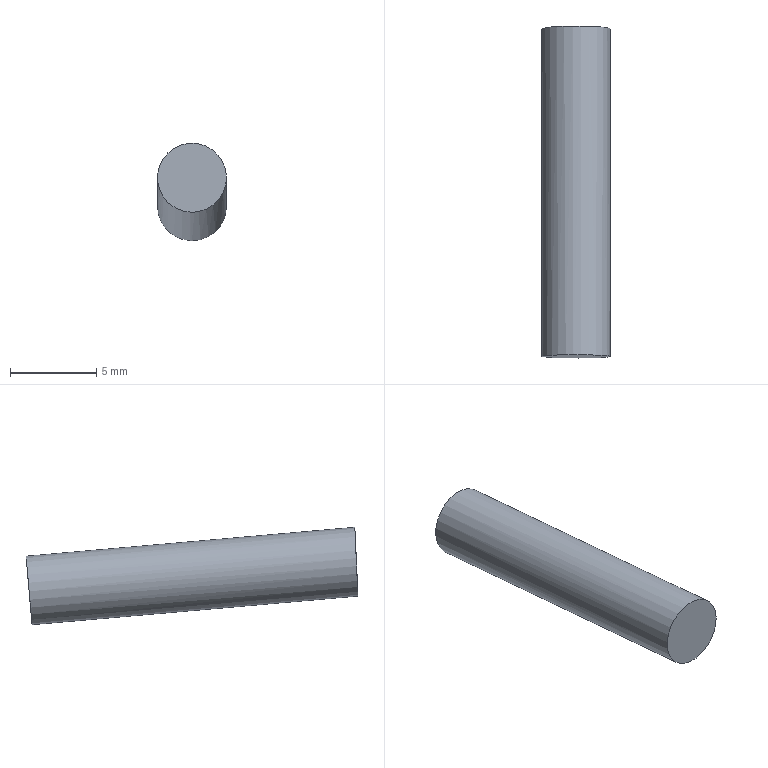Part | NX | features solid 2 | 1 solid | 3 faces | box 4 x 19.25 x 5.653 mm | volume 239.475 mm3 | plane 2 | cylinder 1 | commonest cylinder face diameters 4 x1
STEP:
#1=CARTESIAN_POINT('',(198.727,-27.661,-42.857));
#2=VERTEX_POINT('',#1);
#3=CARTESIAN_POINT('',(198.727,-27.486,-40.864));
#4=DIRECTION('',(0.,-0.9962,0.08716));
#5=DIRECTION('',(0.,-0.08716,-0.9962));
#6=AXIS2_PLACEMENT_3D('',#3,#4,#5);
#7=CIRCLE('',#6,2.);
#8=EDGE_CURVE('',#2,#2,#7,.T.);
#9=ORIENTED_EDGE('',*,*,#8,.F.);
#10=EDGE_LOOP('',(#9));
#11=FACE_BOUND('',#10,.T.);
#12=CARTESIAN_POINT('',(198.727,-27.486,-40.864));
#13=DIRECTION('',(0.,0.9962,-0.08716));
#14=DIRECTION('',(0.,0.08716,0.9962));
#15=AXIS2_PLACEMENT_3D('',#12,#13,#14);
#16=PLANE('',#15);
#17=ADVANCED_FACE('',(#11),#16,.T.);
#18=CARTESIAN_POINT('',(198.633,-46.561,-41.201));
#19=VERTEX_POINT('',#18);
#20=CARTESIAN_POINT('',(198.727,-46.471,-39.203));
#21=DIRECTION('',(0.001957,0.999,-0.04546));
#22=DIRECTION('',(-0.04675,-0.04532,-0.9979));
#23=AXIS2_PLACEMENT_3D('',#20,#21,#22);
#24=ELLIPSE('',#23,2.002,2.);
#25=EDGE_CURVE('',#19,#19,#24,.T.);
#26=ORIENTED_EDGE('',*,*,#25,.F.);
#27=EDGE_LOOP('',(#26));
#28=FACE_BOUND('',#27,.T.);
#29=CARTESIAN_POINT('',(128.811,-48.589,-88.763));
#30=DIRECTION('',(0.001957,0.999,-0.04546));
#31=DIRECTION('',(0.06617,0.04523,0.9968));
#32=AXIS2_PLACEMENT_3D('',#29,#30,#31);
#33=PLANE('',#32);
#34=ADVANCED_FACE('',(#28),#33,.F.);
#35=ORIENTED_EDGE('',*,*,#8,.T.);
#36=EDGE_LOOP('',(#35));
#37=FACE_BOUND('',#36,.T.);
#38=ORIENTED_EDGE('',*,*,#25,.T.);
#39=EDGE_LOOP('',(#38));
#40=FACE_BOUND('',#39,.T.);
#41=CARTESIAN_POINT('',(198.727,-47.41,-39.121));
#42=DIRECTION('',(0.,0.9962,-0.08716));
#43=DIRECTION('',(0.,0.08716,0.9962));
#44=AXIS2_PLACEMENT_3D('',#41,#42,#43);
#45=CYLINDRICAL_SURFACE('',#44,2.);
#46=ADVANCED_FACE('',(#37,#40),#45,.T.);
#47=CLOSED_SHELL('',(#17,#34,#46));
#48=MANIFOLD_SOLID_BREP('',#47);
#49=(LENGTH_UNIT()NAMED_UNIT(*)SI_UNIT(.MILLI.,.METRE.));
#50=UNCERTAINTY_MEASURE_WITH_UNIT(LENGTH_MEASURE(0.00001),#49,'','');
#51=(NAMED_UNIT(*)PLANE_ANGLE_UNIT()SI_UNIT($,.RADIAN.));
#52=(NAMED_UNIT(*)SI_UNIT($,.STERADIAN.)SOLID_ANGLE_UNIT());
#53=(GEOMETRIC_REPRESENTATION_CONTEXT(3)GLOBAL_UNCERTAINTY_ASSIGNED_CONTEXT((#50))GLOBAL_UNIT_ASSIGNED_CONTEXT((#49,#51,#52))REPRESENTATION_CONTEXT('',''));
#54=ADVANCED_BREP_SHAPE_REPRESENTATION('',(#48),#53);